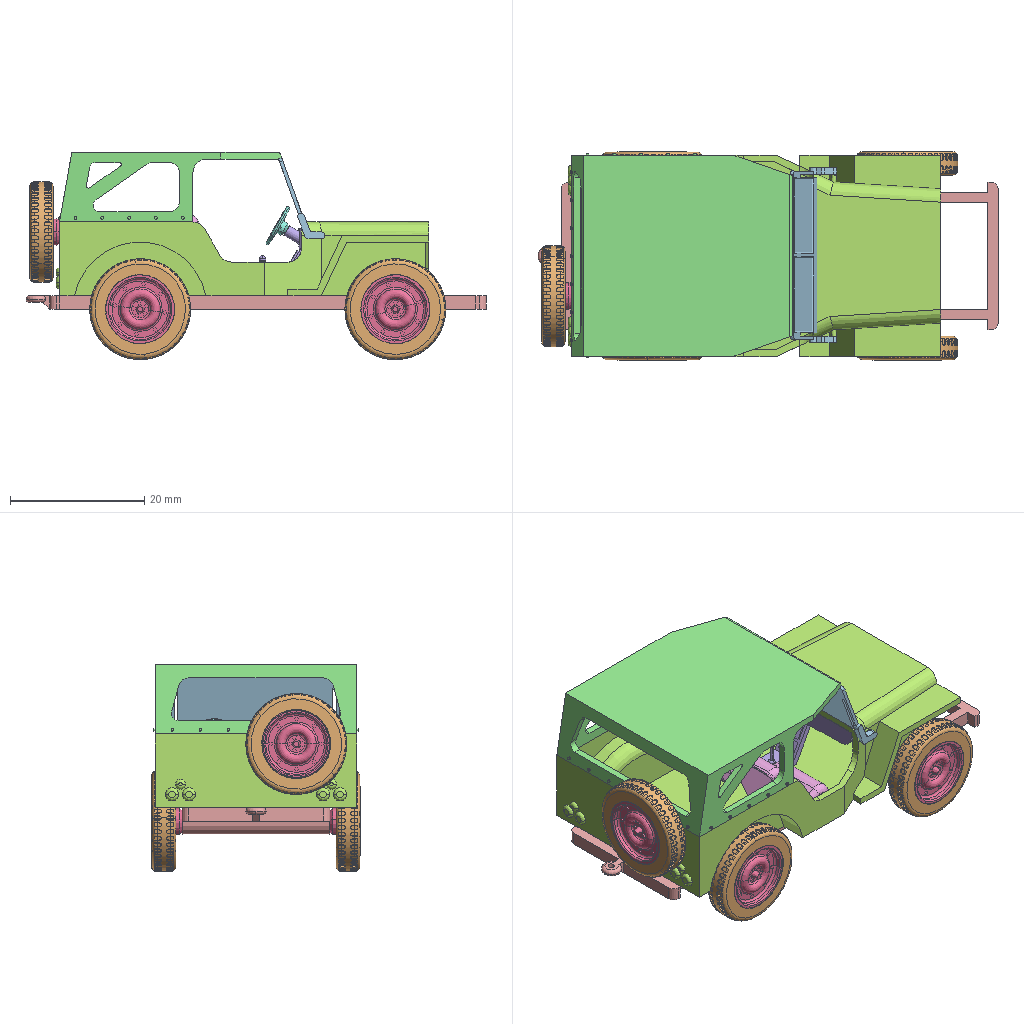Assembly | SolidWorks | 13 different items | 23 placed | box 68 x 31 x 31 mm
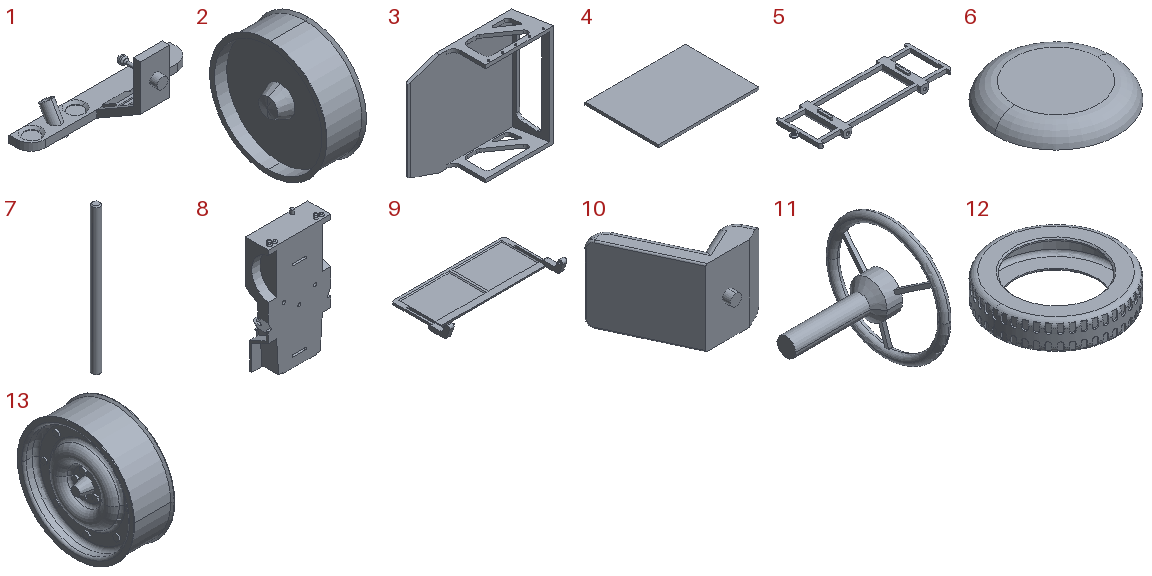Parts list (item | quantity | size | volume | features):
1 | x1 | 21.97 x 10.4 x 10.607 mm | 112.085 mm3 | features ICE 5, Revolution 2, Chamfer 1, Extrusion 1, MirrorPattern 1
2 | x1 | 4.55 x 10.02 x 10.02 mm | 110.565 mm3 | features Revolution 1
3 | x1 | 33.181 x 10.34 x 30.4 mm | 1217 mm3 | features ICE 5, Extrusion 1, MirrorPattern 1, Shell 1
4 | x1 | 11.25 x 8.29 x 0.3 mm | 27.979 mm3 | features Extrusion 1
5 | x1 | 68.5 x 22 x 5 mm | 1025 mm3 | features ICE 7, Extrusion 1, Fillet 1
6 | x1 | 3 x 3 x 0.4 mm | 0.8046 mm3 | features Extrusion 1, Fillet 1, Shell 1
7 | x2 | 1.5 x 1.5 x 27.5 mm | 48.425 mm3 | features Chamfer 1, Extrusion 1
8 | x1 | 30 x 11 x 57 mm | 3381 mm3 | features ICE 10, MirrorPattern 5, Fillet 3, Cut 2, Extrusion 1, Shell 1
9 | x1 | 26.09 x 13.404 x 2.879 mm | 97.812 mm3 | features ICE 4, CutThin 2, Chamfer 1, Extrusion 1, Fillet 1, MirrorPattern 1
10 | x2 | 13.131 x 12.274 x 10 mm | 457.95 mm3 | features Fillet 2, Extrusion 1, ICE 1
11 | x1 | 5.75 x 6.5 x 6.5 mm | 10.173 mm3 | features ICE 2, CirPattern 1, Fillet 1, Revolution 1
12 | x5 | 15 x 15 x 3.5 mm | 81.767 mm3 | features Chamfer 1, CirPattern 1, Extrusion 1, Fillet 1, ICE 1, Shell 1
13 | x5 | 4.55 x 10.3 x 10.3 mm | 146.742 mm3 | features Chamfer 2, CirPattern 2, ICE 2, Fillet 1, Revolution 1
Mates (type | each side: item.copy, entity, surface, feature):
Concentric | 13.1 face cylinder Revolve1 | 12.1 edge
Coincident | 12.1 face plane Boss-Extrude1 | 13.1 face plane Revolve1
Concentric | 5.1 face cylinder Cut-Extrude4 | 7.1 face cylinder Boss-Extrude1
DistanceDim | 5.1 face plane Boss-Extrude1 | 7.1 face plane Boss-Extrude1
Concentric | 7.1 face cylinder Boss-Extrude1 | 13.1 face cylinder Revolve1
Coincident | 5.1 face plane Boss-Extrude1 | 13.1 face plane Revolve1
Concentric | 13.2 edge | 12.2 edge
Coincident | 13.2 face plane Revolve1 | 12.2 face plane Boss-Extrude1
Concentric | 13.3 edge | 12.3 edge
Coincident | 13.3 face plane Revolve1 | 12.3 face plane Boss-Extrude1
Coincident | 13.4 edge | 12.4 edge
Concentric | 5.1 face cylinder Cut-Extrude4 | 7.2 face cylinder Boss-Extrude1
DistanceDim | 7.2 face plane Boss-Extrude1 | 5.1 face plane Boss-Extrude1
Concentric | 13.2 face cylinder Revolve1 | 7.2 face cylinder Boss-Extrude1
Coincident | 5.1 face plane Boss-Extrude1 | 13.2 face plane Revolve1
Concentric | 13.4 face cylinder Revolve1 | 7.2 face cylinder Boss-Extrude1
Coincident | 5.1 face plane Boss-Extrude1 | 13.4 face plane Revolve1
Concentric | 7.1 face cylinder Boss-Extrude1 | 13.3 face cylinder Revolve1
Coincident | 5.1 face plane Boss-Extrude1 | 13.3 face plane Revolve1
Concentric | 8.1 face cylinder Cut-Extrude2 | 12.3 face cylinder Boss-Extrude1
Coincident | 5.1 face plane Boss-Extrude1 | 8.1 face plane Boss-Extrude1
Concentric | 5.1 face cylinder Boss-Extrude3 | 8.1 face cylinder Cut-Extrude7
Concentric | 8.1 face cylinder Cut-Extrude7 | 1.1 face cylinder Revolve2
Coincident | 8.1 face plane Shell6 | 1.1 face plane Boss-Extrude2
Concentric | 8.1 face cylinder Cut-Extrude7 | 10.1 face cylinder Boss-Extrude2
Coincident | 8.1 face plane Shell6 | 10.1 face plane Boss-Extrude1
Parallel | 8.1 face plane Shell6 | 10.1 face plane Boss-Extrude1
Concentric | 8.1 face cylinder Cut-Extrude7 | 10.2 face cylinder Boss-Extrude2
Coincident | 8.1 face plane Shell6 | 10.2 face plane Boss-Extrude1
Parallel | 8.1 face plane Shell6 | 10.2 face plane Boss-Extrude1
Concentric | 11.1 face cylinder Revolve2 | 1.1 face cylinder Cut-Extrude3
Coincident | 11.1 edge | 1.1 face plane Revolve1
Coincident | 8.1 face plane Boss-Extrude1 | 3.1 face plane Boss-Extrude2
Coincident | 8.1 edge | 3.1 edge | 2 times
Coincident | 3.1 edge | 9.1 edge
Coincident | 8.1 edge | 9.1 edge
DistanceDim | 8.1 face plane Boss-Extrude2 | 9.1 face plane Boss-Extrude6
Concentric | 13.5 edge | 12.5 edge
Concentric | 8.1 face cylinder Boss-Extrude4 | 13.5 face cylinder Revolve1
Coincident | 13.5 face plane Revolve1 | 12.5 face plane Boss-Extrude1
Coincident | 8.1 face plane Boss-Extrude1 | 13.5 face plane Revolve1